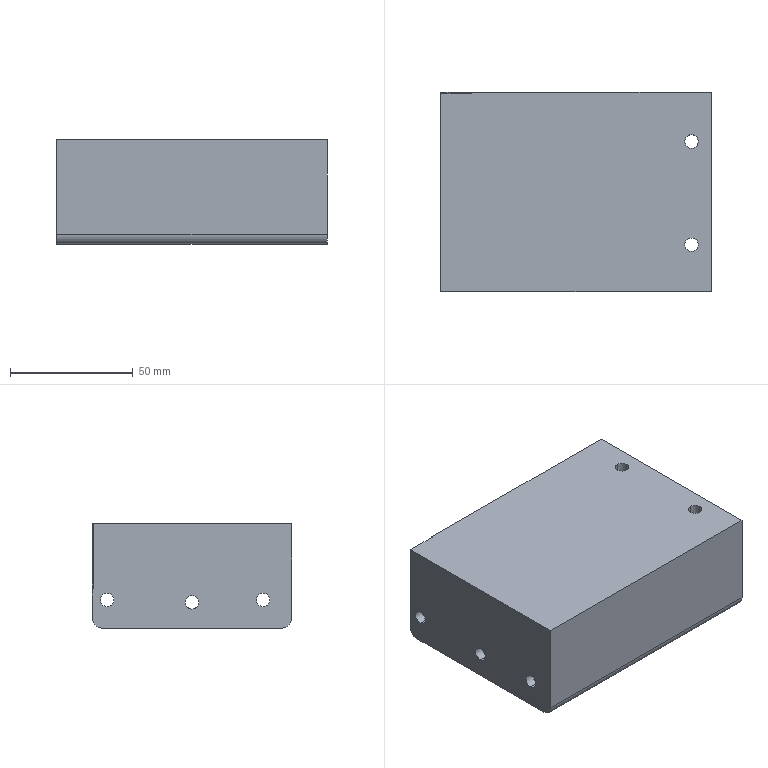Part | STEP file | FFH80-GY-002B^FFH85-PL-M75-B3-01_three-axis module | 1 solid | 46 faces | box 110 x 81 x 42.5 mm | volume 366642 mm3 | cylinder 29 | plane 15 | cone 2 | commonest cylinder face diameters 5.5 x10 9 x10 2.5 x2 3 x2 3.3 x2 8 x2
STEP:
#1=CARTESIAN_POINT('',(102.,23.25,21.25));
#2=VERTEX_POINT('',#1);
#3=CARTESIAN_POINT('',(102.,17.75,21.25));
#4=VERTEX_POINT('',#3);
#5=CARTESIAN_POINT('',(102.,20.5,21.25));
#6=DIRECTION('',(0.,0.,1.));
#7=DIRECTION('',(0.,1.,0.));
#8=AXIS2_PLACEMENT_3D('',#5,#6,#7);
#9=CIRCLE('',#8,2.75);
#10=EDGE_CURVE('',#2,#4,#9,.T.);
#11=ORIENTED_EDGE('',*,*,#10,.T.);
#12=CARTESIAN_POINT('',(102.,17.75,-15.25));
#13=VERTEX_POINT('',#12);
#14=CARTESIAN_POINT('',(102.,17.75,-21.25));
#15=DIRECTION('',(0.,0.,-1.));
#16=VECTOR('',#15,1000.);
#17=LINE('',#14,#16);
#18=EDGE_CURVE('',#4,#13,#17,.T.);
#19=ORIENTED_EDGE('',*,*,#18,.T.);
#20=CARTESIAN_POINT('',(102.,23.25,-15.25));
#21=VERTEX_POINT('',#20);
#22=CARTESIAN_POINT('',(102.,20.5,-15.25));
#23=DIRECTION('',(0.,0.,1.));
#24=DIRECTION('',(0.,1.,0.));
#25=AXIS2_PLACEMENT_3D('',#22,#23,#24);
#26=CIRCLE('',#25,2.75);
#27=EDGE_CURVE('',#21,#13,#26,.T.);
#28=ORIENTED_EDGE('',*,*,#27,.F.);
#29=CARTESIAN_POINT('',(102.,23.25,-21.25));
#30=DIRECTION('',(0.,0.,-1.));
#31=VECTOR('',#30,1000.);
#32=LINE('',#29,#31);
#33=EDGE_CURVE('',#2,#21,#32,.T.);
#34=ORIENTED_EDGE('',*,*,#33,.F.);
#35=EDGE_LOOP('',(#11,#19,#28,#34));
#36=FACE_OUTER_BOUND('',#35,.T.);
#37=CARTESIAN_POINT('',(102.,20.5,-21.25));
#38=DIRECTION('',(0.,0.,-1.));
#39=DIRECTION('',(0.,1.,0.));
#40=AXIS2_PLACEMENT_3D('',#37,#38,#39);
#41=CYLINDRICAL_SURFACE('',#40,2.75);
#42=ADVANCED_FACE('',(#36),#41,.F.);
#43=CARTESIAN_POINT('',(102.,-18.75,21.25));
#44=VERTEX_POINT('',#43);
#45=CARTESIAN_POINT('',(102.,-24.25,21.25));
#46=VERTEX_POINT('',#45);
#47=CARTESIAN_POINT('',(102.,-21.5,21.25));
#48=DIRECTION('',(0.,0.,1.));
#49=DIRECTION('',(0.,1.,0.));
#50=AXIS2_PLACEMENT_3D('',#47,#48,#49);
#51=CIRCLE('',#50,2.75);
#52=EDGE_CURVE('',#44,#46,#51,.T.);
#53=ORIENTED_EDGE('',*,*,#52,.T.);
#54=CARTESIAN_POINT('',(102.,-24.25,-15.25));
#55=VERTEX_POINT('',#54);
#56=CARTESIAN_POINT('',(102.,-24.25,-21.25));
#57=DIRECTION('',(0.,0.,-1.));
#58=VECTOR('',#57,1000.);
#59=LINE('',#56,#58);
#60=EDGE_CURVE('',#46,#55,#59,.T.);
#61=ORIENTED_EDGE('',*,*,#60,.T.);
#62=CARTESIAN_POINT('',(102.,-18.75,-15.25));
#63=VERTEX_POINT('',#62);
#64=CARTESIAN_POINT('',(102.,-21.5,-15.25));
#65=DIRECTION('',(0.,0.,1.));
#66=DIRECTION('',(0.,1.,0.));
#67=AXIS2_PLACEMENT_3D('',#64,#65,#66);
#68=CIRCLE('',#67,2.75);
#69=EDGE_CURVE('',#63,#55,#68,.T.);
#70=ORIENTED_EDGE('',*,*,#69,.F.);
#71=CARTESIAN_POINT('',(102.,-18.75,-21.25));
#72=DIRECTION('',(0.,0.,-1.));
#73=VECTOR('',#72,1000.);
#74=LINE('',#71,#73);
#75=EDGE_CURVE('',#44,#63,#74,.T.);
#76=ORIENTED_EDGE('',*,*,#75,.F.);
#77=EDGE_LOOP('',(#53,#61,#70,#76));
#78=FACE_OUTER_BOUND('',#77,.T.);
#79=CARTESIAN_POINT('',(102.,-21.5,-21.25));
#80=DIRECTION('',(0.,0.,-1.));
#81=DIRECTION('',(0.,1.,0.));
#82=AXIS2_PLACEMENT_3D('',#79,#80,#81);
#83=CYLINDRICAL_SURFACE('',#82,2.75);
#84=ADVANCED_FACE('',(#78),#83,.F.);
#85=CARTESIAN_POINT('',(6.,34.2,3.75));
#86=VERTEX_POINT('',#85);
#87=CARTESIAN_POINT('',(6.,34.2,6.75));
#88=VERTEX_POINT('',#87);
#89=CARTESIAN_POINT('',(6.,34.2,5.25));
#90=DIRECTION('',(0.,1.,0.));
#91=DIRECTION('',(0.,0.,1.));
#92=AXIS2_PLACEMENT_3D('',#89,#90,#91);
#93=CIRCLE('',#92,1.5);
#94=EDGE_CURVE('',#86,#88,#93,.T.);
#95=ORIENTED_EDGE('',*,*,#94,.F.);
#96=CARTESIAN_POINT('',(6.,40.2,3.75));
#97=VERTEX_POINT('',#96);
#98=CARTESIAN_POINT('',(6.,40.2,3.75));
#99=DIRECTION('',(0.,1.,0.));
#100=VECTOR('',#99,1000.);
#101=LINE('',#98,#100);
#102=EDGE_CURVE('',#86,#97,#101,.T.);
#103=ORIENTED_EDGE('',*,*,#102,.T.);
#104=CARTESIAN_POINT('',(6.,40.2,6.75));
#105=VERTEX_POINT('',#104);
#106=CARTESIAN_POINT('',(6.,40.2,5.25));
#107=DIRECTION('',(0.,1.,0.));
#108=DIRECTION('',(0.,0.,1.));
#109=AXIS2_PLACEMENT_3D('',#106,#107,#108);
#110=CIRCLE('',#109,1.5);
#111=EDGE_CURVE('',#97,#105,#110,.T.);
#112=ORIENTED_EDGE('',*,*,#111,.T.);
#113=CARTESIAN_POINT('',(6.,40.2,6.75));
#114=DIRECTION('',(0.,1.,0.));
#115=VECTOR('',#114,1000.);
#116=LINE('',#113,#115);
#117=EDGE_CURVE('',#88,#105,#116,.T.);
#118=ORIENTED_EDGE('',*,*,#117,.F.);
#119=EDGE_LOOP('',(#95,#103,#112,#118));
#120=FACE_OUTER_BOUND('',#119,.T.);
#121=CARTESIAN_POINT('',(6.,40.2,5.25));
#122=DIRECTION('',(0.,1.,0.));
#123=DIRECTION('',(0.,0.,1.));
#124=AXIS2_PLACEMENT_3D('',#121,#122,#123);
#125=CYLINDRICAL_SURFACE('',#124,1.5);
#126=ADVANCED_FACE('',(#120),#125,.F.);
#127=CARTESIAN_POINT('',(0.,0.,-8.));
#128=VERTEX_POINT('',#127);
#129=CARTESIAN_POINT('',(0.,0.,-13.5));
#130=VERTEX_POINT('',#129);
#131=CARTESIAN_POINT('',(0.,0.,-10.75));
#132=DIRECTION('',(1.,0.,0.));
#133=DIRECTION('',(0.,0.,-1.));
#134=AXIS2_PLACEMENT_3D('',#131,#132,#133);
#135=CIRCLE('',#134,2.75);
#136=EDGE_CURVE('',#128,#130,#135,.T.);
#137=ORIENTED_EDGE('',*,*,#136,.F.);
#138=CARTESIAN_POINT('',(104.,0.,-8.));
#139=VERTEX_POINT('',#138);
#140=CARTESIAN_POINT('',(110.,0.,-8.));
#141=DIRECTION('',(1.,0.,0.));
#142=VECTOR('',#141,1000.);
#143=LINE('',#140,#142);
#144=EDGE_CURVE('',#128,#139,#143,.T.);
#145=ORIENTED_EDGE('',*,*,#144,.T.);
#146=CARTESIAN_POINT('',(104.,0.,-13.5));
#147=VERTEX_POINT('',#146);
#148=CARTESIAN_POINT('',(104.,0.,-10.75));
#149=DIRECTION('',(-1.,0.,0.));
#150=DIRECTION('',(0.,0.,-1.));
#151=AXIS2_PLACEMENT_3D('',#148,#149,#150);
#152=CIRCLE('',#151,2.75);
#153=EDGE_CURVE('',#147,#139,#152,.T.);
#154=ORIENTED_EDGE('',*,*,#153,.F.);
#155=CARTESIAN_POINT('',(100.65,0.,-13.5));
#156=VERTEX_POINT('',#155);
#157=CARTESIAN_POINT('',(110.,0.,-13.5));
#158=DIRECTION('',(1.,0.,0.));
#159=VECTOR('',#158,1000.);
#160=LINE('',#157,#159);
#161=EDGE_CURVE('',#156,#147,#160,.T.);
#162=ORIENTED_EDGE('',*,*,#161,.F.);
#163=CARTESIAN_POINT('',(99.,-1.65,-12.95));
#164=VERTEX_POINT('',#163);
#165=CARTESIAN_POINT('',(99.,-1.65,-12.95));
#166=CARTESIAN_POINT('',(99.112,-1.65,-12.95));
#167=CARTESIAN_POINT('',(99.222,-1.639,-12.959));
#168=CARTESIAN_POINT('',(99.436,-1.595,-12.99));
#169=CARTESIAN_POINT('',(99.542,-1.562,-13.014));
#170=CARTESIAN_POINT('',(99.838,-1.437,-13.097));
#171=CARTESIAN_POINT('',(100.016,-1.317,-13.17));
#172=CARTESIAN_POINT('',(100.239,-1.094,-13.274));
#173=CARTESIAN_POINT('',(100.308,-1.012,-13.309));
#174=CARTESIAN_POINT('',(100.427,-0.8358,-13.372));
#175=CARTESIAN_POINT('',(100.477,-0.7424,-13.4));
#176=CARTESIAN_POINT('',(100.562,-0.5439,-13.448));
#177=CARTESIAN_POINT('',(100.595,-0.4374,-13.467));
#178=CARTESIAN_POINT('',(100.639,-0.222,-13.493));
#179=CARTESIAN_POINT('',(100.65,-0.1122,-13.5));
#180=CARTESIAN_POINT('',(100.65,0.,-13.5));
#181=B_SPLINE_CURVE_WITH_KNOTS('',3,(#165,#166,#167,#168,#169,#170,#171,#172,#173,#174,#175,#176,#177,#178,#179,#180),.UNSPECIFIED.,.F.,.F.,(4,2,2,2,2,2,2,4),(0.,0.0003309,0.0006617,0.001323,0.001654,0.001985,0.002316,0.002647),.UNSPECIFIED.);
#182=EDGE_CURVE('',#164,#156,#181,.T.);
#183=ORIENTED_EDGE('',*,*,#182,.F.);
#184=CARTESIAN_POINT('',(97.35,0.,-13.5));
#185=VERTEX_POINT('',#184);
#186=CARTESIAN_POINT('',(97.35,0.,-13.5));
#187=CARTESIAN_POINT('',(97.35,-0.1121,-13.5));
#188=CARTESIAN_POINT('',(97.361,-0.2218,-13.493));
#189=CARTESIAN_POINT('',(97.405,-0.4369,-13.467));
#190=CARTESIAN_POINT('',(97.438,-0.5432,-13.448));
#191=CARTESIAN_POINT('',(97.565,-0.842,-13.376));
#192=CARTESIAN_POINT('',(97.687,-1.021,-13.309));
#193=CARTESIAN_POINT('',(97.91,-1.243,-13.204));
#194=CARTESIAN_POINT('',(97.993,-1.311,-13.168));
#195=CARTESIAN_POINT('',(98.168,-1.429,-13.101));
#196=CARTESIAN_POINT('',(98.261,-1.479,-13.069));
#197=CARTESIAN_POINT('',(98.458,-1.562,-13.014));
#198=CARTESIAN_POINT('',(98.564,-1.595,-12.99));
#199=CARTESIAN_POINT('',(98.778,-1.639,-12.959));
#200=CARTESIAN_POINT('',(98.888,-1.65,-12.95));
#201=CARTESIAN_POINT('',(99.,-1.65,-12.95));
#202=B_SPLINE_CURVE_WITH_KNOTS('',3,(#186,#187,#188,#189,#190,#191,#192,#193,#194,#195,#196,#197,#198,#199,#200,#201),.UNSPECIFIED.,.F.,.F.,(4,2,2,2,2,2,2,4),(-0.002649,-0.002318,-0.001986,-0.001324,-0.0009932,-0.0006622,-0.0003311,0.),.UNSPECIFIED.);
#203=EDGE_CURVE('',#185,#164,#202,.T.);
#204=ORIENTED_EDGE('',*,*,#203,.F.);
#205=CARTESIAN_POINT('',(110.,0.,-13.5));
#206=DIRECTION('',(1.,0.,0.));
#207=VECTOR('',#206,1000.);
#208=LINE('',#205,#207);
#209=EDGE_CURVE('',#130,#185,#208,.T.);
#210=ORIENTED_EDGE('',*,*,#209,.F.);
#211=EDGE_LOOP('',(#137,#145,#154,#162,#183,#204,#210));
#212=FACE_OUTER_BOUND('',#211,.T.);
#213=CARTESIAN_POINT('',(110.,0.,-10.75));
#214=DIRECTION('',(1.,0.,0.));
#215=DIRECTION('',(0.,0.,-1.));
#216=AXIS2_PLACEMENT_3D('',#213,#214,#215);
#217=CYLINDRICAL_SURFACE('',#216,2.75);
#218=ADVANCED_FACE('',(#212),#217,.F.);
#219=CARTESIAN_POINT('',(0.,34.5,-7.));
#220=VERTEX_POINT('',#219);
#221=CARTESIAN_POINT('',(0.,34.5,-12.5));
#222=VERTEX_POINT('',#221);
#223=CARTESIAN_POINT('',(0.,34.5,-9.75));
#224=DIRECTION('',(1.,0.,0.));
#225=DIRECTION('',(0.,0.,-1.));
#226=AXIS2_PLACEMENT_3D('',#223,#224,#225);
#227=CIRCLE('',#226,2.75);
#228=EDGE_CURVE('',#220,#222,#227,.T.);
#229=ORIENTED_EDGE('',*,*,#228,.F.);
#230=CARTESIAN_POINT('',(104.,34.5,-7.));
#231=VERTEX_POINT('',#230);
#232=CARTESIAN_POINT('',(110.,34.5,-7.));
#233=DIRECTION('',(1.,0.,0.));
#234=VECTOR('',#233,1000.);
#235=LINE('',#232,#234);
#236=EDGE_CURVE('',#220,#231,#235,.T.);
#237=ORIENTED_EDGE('',*,*,#236,.T.);
#238=CARTESIAN_POINT('',(104.,34.5,-12.5));
#239=VERTEX_POINT('',#238);
#240=CARTESIAN_POINT('',(104.,34.5,-9.75));
#241=DIRECTION('',(-1.,0.,0.));
#242=DIRECTION('',(0.,0.,-1.));
#243=AXIS2_PLACEMENT_3D('',#240,#241,#242);
#244=CIRCLE('',#243,2.75);
#245=EDGE_CURVE('',#239,#231,#244,.T.);
#246=ORIENTED_EDGE('',*,*,#245,.F.);
#247=CARTESIAN_POINT('',(110.,34.5,-12.5));
#248=DIRECTION('',(1.,0.,0.));
#249=VECTOR('',#248,1000.);
#250=LINE('',#247,#249);
#251=EDGE_CURVE('',#222,#239,#250,.T.);
#252=ORIENTED_EDGE('',*,*,#251,.F.);
#253=EDGE_LOOP('',(#229,#237,#246,#252));
#254=FACE_OUTER_BOUND('',#253,.T.);
#255=CARTESIAN_POINT('',(110.,34.5,-9.75));
#256=DIRECTION('',(1.,0.,0.));
#257=DIRECTION('',(0.,0.,-1.));
#258=AXIS2_PLACEMENT_3D('',#255,#256,#257);
#259=CYLINDRICAL_SURFACE('',#258,2.75);
#260=ADVANCED_FACE('',(#254),#259,.F.);
#261=CARTESIAN_POINT('',(0.,-29.,-7.));
#262=VERTEX_POINT('',#261);
#263=CARTESIAN_POINT('',(0.,-29.,-12.5));
#264=VERTEX_POINT('',#263);
#265=CARTESIAN_POINT('',(0.,-29.,-9.75));
#266=DIRECTION('',(1.,0.,0.));
#267=DIRECTION('',(0.,0.,-1.));
#268=AXIS2_PLACEMENT_3D('',#265,#266,#267);
#269=CIRCLE('',#268,2.75);
#270=EDGE_CURVE('',#262,#264,#269,.T.);
#271=ORIENTED_EDGE('',*,*,#270,.F.);
#272=CARTESIAN_POINT('',(104.,-29.,-7.));
#273=VERTEX_POINT('',#272);
#274=CARTESIAN_POINT('',(110.,-29.,-7.));
#275=DIRECTION('',(1.,0.,0.));
#276=VECTOR('',#275,1000.);
#277=LINE('',#274,#276);
#278=EDGE_CURVE('',#262,#273,#277,.T.);
#279=ORIENTED_EDGE('',*,*,#278,.T.);
#280=CARTESIAN_POINT('',(104.,-29.,-12.5));
#281=VERTEX_POINT('',#280);
#282=CARTESIAN_POINT('',(104.,-29.,-9.75));
#283=DIRECTION('',(-1.,0.,0.));
#284=DIRECTION('',(0.,0.,-1.));
#285=AXIS2_PLACEMENT_3D('',#282,#283,#284);
#286=CIRCLE('',#285,2.75);
#287=EDGE_CURVE('',#281,#273,#286,.T.);
#288=ORIENTED_EDGE('',*,*,#287,.F.);
#289=CARTESIAN_POINT('',(110.,-29.,-12.5));
#290=DIRECTION('',(1.,0.,0.));
#291=VECTOR('',#290,1000.);
#292=LINE('',#289,#291);
#293=EDGE_CURVE('',#264,#281,#292,.T.);
#294=ORIENTED_EDGE('',*,*,#293,.F.);
#295=EDGE_LOOP('',(#271,#279,#288,#294));
#296=FACE_OUTER_BOUND('',#295,.T.);
#297=CARTESIAN_POINT('',(110.,-29.,-9.75));
#298=DIRECTION('',(1.,0.,0.));
#299=DIRECTION('',(0.,0.,-1.));
#300=AXIS2_PLACEMENT_3D('',#297,#298,#299);
#301=CYLINDRICAL_SURFACE('',#300,2.75);
#302=ADVANCED_FACE('',(#296),#301,.F.);
#303=CARTESIAN_POINT('',(104.,0.,-6.25));
#304=VERTEX_POINT('',#303);
#305=CARTESIAN_POINT('',(104.,0.,-15.25));
#306=VERTEX_POINT('',#305);
#307=CARTESIAN_POINT('',(104.,0.,-10.75));
#308=DIRECTION('',(1.,0.,0.));
#309=DIRECTION('',(0.,0.,-1.));
#310=AXIS2_PLACEMENT_3D('',#307,#308,#309);
#311=CIRCLE('',#310,4.5);
#312=EDGE_CURVE('',#304,#306,#311,.T.);
#313=ORIENTED_EDGE('',*,*,#312,.F.);
#314=CARTESIAN_POINT('',(110.,0.,-6.25));
#315=VERTEX_POINT('',#314);
#316=CARTESIAN_POINT('',(110.,0.,-6.25));
#317=DIRECTION('',(1.,0.,0.));
#318=VECTOR('',#317,1000.);
#319=LINE('',#316,#318);
#320=EDGE_CURVE('',#304,#315,#319,.T.);
#321=ORIENTED_EDGE('',*,*,#320,.T.);
#322=CARTESIAN_POINT('',(110.,0.,-15.25));
#323=VERTEX_POINT('',#322);
#324=CARTESIAN_POINT('',(110.,0.,-10.75));
#325=DIRECTION('',(1.,0.,0.));
#326=DIRECTION('',(0.,0.,-1.));
#327=AXIS2_PLACEMENT_3D('',#324,#325,#326);
#328=CIRCLE('',#327,4.5);
#329=EDGE_CURVE('',#315,#323,#328,.T.);
#330=ORIENTED_EDGE('',*,*,#329,.T.);
#331=CARTESIAN_POINT('',(110.,0.,-15.25));
#332=DIRECTION('',(1.,0.,0.));
#333=VECTOR('',#332,1000.);
#334=LINE('',#331,#333);
#335=EDGE_CURVE('',#306,#323,#334,.T.);
#336=ORIENTED_EDGE('',*,*,#335,.F.);
#337=EDGE_LOOP('',(#313,#321,#330,#336));
#338=FACE_OUTER_BOUND('',#337,.T.);
#339=CARTESIAN_POINT('',(110.,0.,-10.75));
#340=DIRECTION('',(1.,0.,0.));
#341=DIRECTION('',(0.,0.,-1.));
#342=AXIS2_PLACEMENT_3D('',#339,#340,#341);
#343=CYLINDRICAL_SURFACE('',#342,4.5);
#344=ADVANCED_FACE('',(#338),#343,.F.);
#345=CARTESIAN_POINT('',(104.,34.5,-5.25));
#346=VERTEX_POINT('',#345);
#347=CARTESIAN_POINT('',(104.,34.5,-14.25));
#348=VERTEX_POINT('',#347);
#349=CARTESIAN_POINT('',(104.,34.5,-9.75));
#350=DIRECTION('',(1.,0.,0.));
#351=DIRECTION('',(0.,0.,-1.));
#352=AXIS2_PLACEMENT_3D('',#349,#350,#351);
#353=CIRCLE('',#352,4.5);
#354=EDGE_CURVE('',#346,#348,#353,.T.);
#355=ORIENTED_EDGE('',*,*,#354,.F.);
#356=CARTESIAN_POINT('',(110.,34.5,-5.25));
#357=VERTEX_POINT('',#356);
#358=CARTESIAN_POINT('',(110.,34.5,-5.25));
#359=DIRECTION('',(1.,0.,0.));
#360=VECTOR('',#359,1000.);
#361=LINE('',#358,#360);
#362=EDGE_CURVE('',#346,#357,#361,.T.);
#363=ORIENTED_EDGE('',*,*,#362,.T.);
#364=CARTESIAN_POINT('',(110.,34.5,-14.25));
#365=VERTEX_POINT('',#364);
#366=CARTESIAN_POINT('',(110.,34.5,-9.75));
#367=DIRECTION('',(1.,0.,0.));
#368=DIRECTION('',(0.,0.,-1.));
#369=AXIS2_PLACEMENT_3D('',#366,#367,#368);
#370=CIRCLE('',#369,4.5);
#371=EDGE_CURVE('',#357,#365,#370,.T.);
#372=ORIENTED_EDGE('',*,*,#371,.T.);
#373=CARTESIAN_POINT('',(110.,34.5,-14.25));
#374=DIRECTION('',(1.,0.,0.));
#375=VECTOR('',#374,1000.);
#376=LINE('',#373,#375);
#377=EDGE_CURVE('',#348,#365,#376,.T.);
#378=ORIENTED_EDGE('',*,*,#377,.F.);
#379=EDGE_LOOP('',(#355,#363,#372,#378));
#380=FACE_OUTER_BOUND('',#379,.T.);
#381=CARTESIAN_POINT('',(110.,34.5,-9.75));
#382=DIRECTION('',(1.,0.,0.));
#383=DIRECTION('',(0.,0.,-1.));
#384=AXIS2_PLACEMENT_3D('',#381,#382,#383);
#385=CYLINDRICAL_SURFACE('',#384,4.5);
#386=ADVANCED_FACE('',(#380),#385,.F.);
#387=CARTESIAN_POINT('',(104.,-29.,-5.25));
#388=VERTEX_POINT('',#387);
#389=CARTESIAN_POINT('',(104.,-29.,-14.25));
#390=VERTEX_POINT('',#389);
#391=CARTESIAN_POINT('',(104.,-29.,-9.75));
#392=DIRECTION('',(1.,0.,0.));
#393=DIRECTION('',(0.,0.,-1.));
#394=AXIS2_PLACEMENT_3D('',#391,#392,#393);
#395=CIRCLE('',#394,4.5);
#396=EDGE_CURVE('',#388,#390,#395,.T.);
#397=ORIENTED_EDGE('',*,*,#396,.F.);
#398=CARTESIAN_POINT('',(110.,-29.,-5.25));
#399=VERTEX_POINT('',#398);
#400=CARTESIAN_POINT('',(110.,-29.,-5.25));
#401=DIRECTION('',(1.,0.,0.));
#402=VECTOR('',#401,1000.);
#403=LINE('',#400,#402);
#404=EDGE_CURVE('',#388,#399,#403,.T.);
#405=ORIENTED_EDGE('',*,*,#404,.T.);
#406=CARTESIAN_POINT('',(110.,-29.,-14.25));
#407=VERTEX_POINT('',#406);
#408=CARTESIAN_POINT('',(110.,-29.,-9.75));
#409=DIRECTION('',(1.,0.,0.));
#410=DIRECTION('',(0.,0.,-1.));
#411=AXIS2_PLACEMENT_3D('',#408,#409,#410);
#412=CIRCLE('',#411,4.5);
#413=EDGE_CURVE('',#399,#407,#412,.T.);
#414=ORIENTED_EDGE('',*,*,#413,.T.);
#415=CARTESIAN_POINT('',(110.,-29.,-14.25));
#416=DIRECTION('',(1.,0.,0.));
#417=VECTOR('',#416,1000.);
#418=LINE('',#415,#417);
#419=EDGE_CURVE('',#390,#407,#418,.T.);
#420=ORIENTED_EDGE('',*,*,#419,.F.);
#421=EDGE_LOOP('',(#397,#405,#414,#420));
#422=FACE_OUTER_BOUND('',#421,.T.);
#423=CARTESIAN_POINT('',(110.,-29.,-9.75));
#424=DIRECTION('',(1.,0.,0.));
#425=DIRECTION('',(0.,0.,-1.));
#426=AXIS2_PLACEMENT_3D('',#423,#424,#425);
#427=CYLINDRICAL_SURFACE('',#426,4.5);
#428=ADVANCED_FACE('',(#422),#427,.F.);
#429=CARTESIAN_POINT('',(102.,25.,-15.25));
#430=VERTEX_POINT('',#429);
#431=CARTESIAN_POINT('',(102.,16.,-15.25));
#432=VERTEX_POINT('',#431);
#433=CARTESIAN_POINT('',(102.,20.5,-15.25));
#434=DIRECTION('',(0.,0.,1.));
#435=DIRECTION('',(0.,1.,0.));
#436=AXIS2_PLACEMENT_3D('',#433,#434,#435);
#437=CIRCLE('',#436,4.5);
#438=EDGE_CURVE('',#430,#432,#437,.T.);
#439=ORIENTED_EDGE('',*,*,#438,.T.);
#440=CARTESIAN_POINT('',(102.,16.,-21.25));
#441=VERTEX_POINT('',#440);
#442=CARTESIAN_POINT('',(102.,16.,-21.25));
#443=DIRECTION('',(0.,0.,-1.));
#444=VECTOR('',#443,1000.);
#445=LINE('',#442,#444);
#446=EDGE_CURVE('',#432,#441,#445,.T.);
#447=ORIENTED_EDGE('',*,*,#446,.T.);
#448=CARTESIAN_POINT('',(102.,25.,-21.25));
#449=VERTEX_POINT('',#448);
#450=CARTESIAN_POINT('',(102.,20.5,-21.25));
#451=DIRECTION('',(0.,0.,-1.));
#452=DIRECTION('',(0.,1.,0.));
#453=AXIS2_PLACEMENT_3D('',#450,#451,#452);
#454=CIRCLE('',#453,4.5);
#455=EDGE_CURVE('',#441,#449,#454,.T.);
#456=ORIENTED_EDGE('',*,*,#455,.T.);
#457=CARTESIAN_POINT('',(102.,25.,-21.25));
#458=DIRECTION('',(0.,0.,-1.));
#459=VECTOR('',#458,1000.);
#460=LINE('',#457,#459);
#461=EDGE_CURVE('',#430,#449,#460,.T.);
#462=ORIENTED_EDGE('',*,*,#461,.F.);
#463=EDGE_LOOP('',(#439,#447,#456,#462));
#464=FACE_OUTER_BOUND('',#463,.T.);
#465=CARTESIAN_POINT('',(102.,20.5,-21.25));
#466=DIRECTION('',(0.,0.,-1.));
#467=DIRECTION('',(0.,1.,0.));
#468=AXIS2_PLACEMENT_3D('',#465,#466,#467);
#469=CYLINDRICAL_SURFACE('',#468,4.5);
#470=ADVANCED_FACE('',(#464),#469,.F.);
#471=CARTESIAN_POINT('',(102.,-17.,-15.25));
#472=VERTEX_POINT('',#471);
#473=CARTESIAN_POINT('',(102.,-26.,-15.25));
#474=VERTEX_POINT('',#473);
#475=CARTESIAN_POINT('',(102.,-21.5,-15.25));
#476=DIRECTION('',(0.,0.,1.));
#477=DIRECTION('',(0.,1.,0.));
#478=AXIS2_PLACEMENT_3D('',#475,#476,#477);
#479=CIRCLE('',#478,4.5);
#480=EDGE_CURVE('',#472,#474,#479,.T.);
#481=ORIENTED_EDGE('',*,*,#480,.T.);
#482=CARTESIAN_POINT('',(102.,-26.,-21.25));
#483=VERTEX_POINT('',#482);
#484=CARTESIAN_POINT('',(102.,-26.,-21.25));
#485=DIRECTION('',(0.,0.,-1.));
#486=VECTOR('',#485,1000.);
#487=LINE('',#484,#486);
#488=EDGE_CURVE('',#474,#483,#487,.T.);
#489=ORIENTED_EDGE('',*,*,#488,.T.);
#490=CARTESIAN_POINT('',(102.,-17.,-21.25));
#491=VERTEX_POINT('',#490);
#492=CARTESIAN_POINT('',(102.,-21.5,-21.25));
#493=DIRECTION('',(0.,0.,-1.));
#494=DIRECTION('',(0.,1.,0.));
#495=AXIS2_PLACEMENT_3D('',#492,#493,#494);
#496=CIRCLE('',#495,4.5);
#497=EDGE_CURVE('',#483,#491,#496,.T.);
#498=ORIENTED_EDGE('',*,*,#497,.T.);
#499=CARTESIAN_POINT('',(102.,-17.,-21.25));
#500=DIRECTION('',(0.,0.,-1.));
#501=VECTOR('',#500,1000.);
#502=LINE('',#499,#501);
#503=EDGE_CURVE('',#472,#491,#502,.T.);
#504=ORIENTED_EDGE('',*,*,#503,.F.);
#505=EDGE_LOOP('',(#481,#489,#498,#504));
#506=FACE_OUTER_BOUND('',#505,.T.);
#507=CARTESIAN_POINT('',(102.,-21.5,-21.25));
#508=DIRECTION('',(0.,0.,-1.));
#509=DIRECTION('',(0.,1.,0.));
#510=AXIS2_PLACEMENT_3D('',#507,#508,#509);
#511=CYLINDRICAL_SURFACE('',#510,4.5);
#512=ADVANCED_FACE('',(#506),#511,.F.);
#513=CARTESIAN_POINT('',(99.,1.65,-12.95));
#514=VERTEX_POINT('',#513);
#515=CARTESIAN_POINT('',(99.,1.65,-12.95));
#516=CARTESIAN_POINT('',(98.888,1.65,-12.95));
#517=CARTESIAN_POINT('',(98.778,1.639,-12.959));
#518=CARTESIAN_POINT('',(98.564,1.595,-12.99));
#519=CARTESIAN_POINT('',(98.458,1.562,-13.014));
#520=CARTESIAN_POINT('',(98.162,1.437,-13.097));
#521=CARTESIAN_POINT('',(97.984,1.317,-13.17));
#522=CARTESIAN_POINT('',(97.761,1.094,-13.274));
#523=CARTESIAN_POINT('',(97.692,1.012,-13.309));
#524=CARTESIAN_POINT('',(97.573,0.8358,-13.372));
#525=CARTESIAN_POINT('',(97.523,0.7424,-13.4));
#526=CARTESIAN_POINT('',(97.438,0.5439,-13.448));
#527=CARTESIAN_POINT('',(97.405,0.4374,-13.467));
#528=CARTESIAN_POINT('',(97.361,0.222,-13.493));
#529=CARTESIAN_POINT('',(97.35,0.1119,-13.5));
#530=CARTESIAN_POINT('',(97.35,0.,-13.5));
#531=B_SPLINE_CURVE_WITH_KNOTS('',3,(#515,#516,#517,#518,#519,#520,#521,#522,#523,#524,#525,#526,#527,#528,#529,#530),.UNSPECIFIED.,.F.,.F.,(4,2,2,2,2,2,2,4),(0.005292,0.005622,0.005953,0.006614,0.006944,0.007274,0.007605,0.007935),.UNSPECIFIED.);
#532=EDGE_CURVE('',#514,#185,#531,.T.);
#533=ORIENTED_EDGE('',*,*,#532,.T.);
#534=ORIENTED_EDGE('',*,*,#203,.T.);
#535=CARTESIAN_POINT('',(99.,-1.65,-21.25));
#536=VERTEX_POINT('',#535);
#537=CARTESIAN_POINT('',(99.,-1.65,-21.25));
#538=DIRECTION('',(0.,0.,-1.));
#539=VECTOR('',#538,1000.);
#540=LINE('',#537,#539);
#541=EDGE_CURVE('',#164,#536,#540,.T.);
#542=ORIENTED_EDGE('',*,*,#541,.T.);
#543=CARTESIAN_POINT('',(99.,1.65,-21.25));
#544=VERTEX_POINT('',#543);
#545=CARTESIAN_POINT('',(99.,0.,-21.25));
#546=DIRECTION('',(0.,0.,-1.));
#547=DIRECTION('',(0.,1.,0.));
#548=AXIS2_PLACEMENT_3D('',#545,#546,#547);
#549=CIRCLE('',#548,1.65);
#550=EDGE_CURVE('',#536,#544,#549,.T.);
#551=ORIENTED_EDGE('',*,*,#550,.T.);
#552=CARTESIAN_POINT('',(99.,1.65,-21.25));
#553=DIRECTION('',(0.,0.,-1.));
#554=VECTOR('',#553,1000.);
#555=LINE('',#552,#554);
#556=EDGE_CURVE('',#514,#544,#555,.T.);
#557=ORIENTED_EDGE('',*,*,#556,.F.);
#558=EDGE_LOOP('',(#533,#534,#542,#551,#557));
#559=FACE_OUTER_BOUND('',#558,.T.);
#560=CARTESIAN_POINT('',(99.,0.,-21.25));
#561=DIRECTION('',(0.,0.,-1.));
#562=DIRECTION('',(0.,1.,0.));
#563=AXIS2_PLACEMENT_3D('',#560,#561,#562);
#564=CYLINDRICAL_SURFACE('',#563,1.65);
#565=ADVANCED_FACE('',(#559),#564,.F.);
#566=CARTESIAN_POINT('',(6.,31.7,4.));
#567=VERTEX_POINT('',#566);
#568=CARTESIAN_POINT('',(6.,31.7,6.5));
#569=VERTEX_POINT('',#568);
#570=CARTESIAN_POINT('',(6.,31.7,5.25));
#571=DIRECTION('',(0.,1.,0.));
#572=DIRECTION('',(0.,0.,1.));
#573=AXIS2_PLACEMENT_3D('',#570,#571,#572);
#574=CIRCLE('',#573,1.25);
#575=EDGE_CURVE('',#567,#569,#574,.T.);
#576=ORIENTED_EDGE('',*,*,#575,.F.);
#577=CARTESIAN_POINT('',(6.,34.2,4.));
#578=VERTEX_POINT('',#577);
#579=CARTESIAN_POINT('',(6.,40.2,4.));
#580=DIRECTION('',(0.,1.,0.));
#581=VECTOR('',#580,1000.);
#582=LINE('',#579,#581);
#583=EDGE_CURVE('',#567,#578,#582,.T.);
#584=ORIENTED_EDGE('',*,*,#583,.T.);
#585=CARTESIAN_POINT('',(6.,34.2,6.5));
#586=VERTEX_POINT('',#585);
#587=CARTESIAN_POINT('',(6.,34.2,5.25));
#588=DIRECTION('',(0.,1.,0.));
#589=DIRECTION('',(0.,0.,1.));
#590=AXIS2_PLACEMENT_3D('',#587,#588,#589);
#591=CIRCLE('',#590,1.25);
#592=EDGE_CURVE('',#578,#586,#591,.T.);
#593=ORIENTED_EDGE('',*,*,#592,.T.);
#594=CARTESIAN_POINT('',(6.,40.2,6.5));
#595=DIRECTION('',(0.,1.,0.));
#596=VECTOR('',#595,1000.);
#597=LINE('',#594,#596);
#598=EDGE_CURVE('',#569,#586,#597,.T.);
#599=ORIENTED_EDGE('',*,*,#598,.F.);
#600=EDGE_LOOP('',(#576,#584,#593,#599));
#601=FACE_OUTER_BOUND('',#600,.T.);
#602=CARTESIAN_POINT('',(6.,40.2,5.25));
#603=DIRECTION('',(0.,1.,0.));
#604=DIRECTION('',(0.,0.,1.));
#605=AXIS2_PLACEMENT_3D('',#602,#603,#604);
#606=CYLINDRICAL_SURFACE('',#605,1.25);
#607=ADVANCED_FACE('',(#601),#606,.F.);
#608=CARTESIAN_POINT('',(6.,30.949,5.25));
#609=VERTEX_POINT('',#608);
#610=CARTESIAN_POINT('',(6.,31.7,6.5));
#611=DIRECTION('',(0.,0.515,0.8572));
#612=VECTOR('',#611,1000.);
#613=LINE('',#610,#612);
#614=EDGE_CURVE('',#609,#569,#613,.T.);
#615=ORIENTED_EDGE('',*,*,#614,.F.);
#616=CARTESIAN_POINT('',(6.,31.7,4.));
#617=DIRECTION('',(0.,0.515,-0.8572));
#618=VECTOR('',#617,1000.);
#619=LINE('',#616,#618);
#620=EDGE_CURVE('',#609,#567,#619,.T.);
#621=ORIENTED_EDGE('',*,*,#620,.T.);
#622=ORIENTED_EDGE('',*,*,#575,.T.);
#623=EDGE_LOOP('',(#615,#621,#622));
#624=FACE_OUTER_BOUND('',#623,.T.);
#625=CARTESIAN_POINT('',(6.,31.7,5.25));
#626=DIRECTION('',(0.,1.,0.));
#627=DIRECTION('',(0.,0.,1.));
#628=AXIS2_PLACEMENT_3D('',#625,#626,#627);
#629=CONICAL_SURFACE('',#628,1.25,1.03);
#630=ADVANCED_FACE('',(#624),#629,.F.);
#631=ORIENTED_EDGE('',*,*,#10,.F.);
#632=CARTESIAN_POINT('',(102.,20.5,21.25));
#633=DIRECTION('',(0.,0.,1.));
#634=DIRECTION('',(0.,1.,0.));
#635=AXIS2_PLACEMENT_3D('',#632,#633,#634);
#636=CIRCLE('',#635,2.75);
#637=EDGE_CURVE('',#4,#2,#636,.T.);
#638=ORIENTED_EDGE('',*,*,#637,.F.);
#639=EDGE_LOOP('',(#631,#638));
#640=FACE_BOUND('',#639,.T.);
#641=ORIENTED_EDGE('',*,*,#52,.F.);
#642=CARTESIAN_POINT('',(102.,-21.5,21.25));
#643=DIRECTION('',(0.,0.,1.));
#644=DIRECTION('',(0.,1.,0.));
#645=AXIS2_PLACEMENT_3D('',#642,#643,#644);
#646=CIRCLE('',#645,2.75);
#647=EDGE_CURVE('',#46,#44,#646,.T.);
#648=ORIENTED_EDGE('',*,*,#647,.F.);
#649=EDGE_LOOP('',(#641,#648));
#650=FACE_BOUND('',#649,.T.);
#651=CARTESIAN_POINT('',(0.,40.2,21.25));
#652=VERTEX_POINT('',#651);
#653=CARTESIAN_POINT('',(12.5,40.2,21.25));
#654=VERTEX_POINT('',#653);
#655=CARTESIAN_POINT('',(110.,40.2,21.25));
#656=DIRECTION('',(1.,0.,0.));
#657=VECTOR('',#656,1000.);
#658=LINE('',#655,#657);
#659=EDGE_CURVE('',#652,#654,#658,.T.);
#660=ORIENTED_EDGE('',*,*,#659,.F.);
#661=CARTESIAN_POINT('',(0.,-40.5,21.25));
#662=VERTEX_POINT('',#661);
#663=CARTESIAN_POINT('',(0.,40.5,21.25));
#664=DIRECTION('',(0.,1.,0.));
#665=VECTOR('',#664,1000.);
#666=LINE('',#663,#665);
#667=EDGE_CURVE('',#662,#652,#666,.T.);
#668=ORIENTED_EDGE('',*,*,#667,.F.);
#669=CARTESIAN_POINT('',(110.,-40.5,21.25));
#670=VERTEX_POINT('',#669);
#671=CARTESIAN_POINT('',(110.,-40.5,21.25));
#672=DIRECTION('',(-1.,0.,0.));
#673=VECTOR('',#672,1000.);
#674=LINE('',#671,#673);
#675=EDGE_CURVE('',#670,#662,#674,.T.);
#676=ORIENTED_EDGE('',*,*,#675,.F.);
#677=CARTESIAN_POINT('',(110.,40.5,21.25));
#678=VERTEX_POINT('',#677);
#679=CARTESIAN_POINT('',(110.,40.5,21.25));
#680=DIRECTION('',(0.,-1.,0.));
#681=VECTOR('',#680,1000.);
#682=LINE('',#679,#681);
#683=EDGE_CURVE('',#678,#670,#682,.T.);
#684=ORIENTED_EDGE('',*,*,#683,.F.);
#685=CARTESIAN_POINT('',(12.5,40.5,21.25));
#686=VERTEX_POINT('',#685);
#687=CARTESIAN_POINT('',(110.,40.5,21.25));
#688=DIRECTION('',(1.,0.,0.));
#689=VECTOR('',#688,1000.);
#690=LINE('',#687,#689);
#691=EDGE_CURVE('',#686,#678,#690,.T.);
#692=ORIENTED_EDGE('',*,*,#691,.F.);
#693=CARTESIAN_POINT('',(12.5,40.2,21.25));
#694=DIRECTION('',(0.,-1.,0.));
#695=VECTOR('',#694,1000.);
#696=LINE('',#693,#695);
#697=EDGE_CURVE('',#686,#654,#696,.T.);
#698=ORIENTED_EDGE('',*,*,#697,.T.);
#699=EDGE_LOOP('',(#660,#668,#676,#684,#692,#698));
#700=FACE_OUTER_BOUND('',#699,.T.);
#701=CARTESIAN_POINT('',(110.,40.5,21.25));
#702=DIRECTION('',(0.,0.,-1.));
#703=DIRECTION('',(-1.,0.,0.));
#704=AXIS2_PLACEMENT_3D('',#701,#702,#703);
#705=PLANE('',#704);
#706=ADVANCED_FACE('',(#640,#650,#700),#705,.F.);
#707=ORIENTED_EDGE('',*,*,#18,.F.);
#708=ORIENTED_EDGE('',*,*,#637,.T.);
#709=ORIENTED_EDGE('',*,*,#33,.T.);
#710=CARTESIAN_POINT('',(102.,20.5,-15.25));
#711=DIRECTION('',(0.,0.,1.));
#712=DIRECTION('',(0.,1.,0.));
#713=AXIS2_PLACEMENT_3D('',#710,#711,#712);
#714=CIRCLE('',#713,2.75);
#715=EDGE_CURVE('',#13,#21,#714,.T.);
#716=ORIENTED_EDGE('',*,*,#715,.F.);
#717=EDGE_LOOP('',(#707,#708,#709,#716));
#718=FACE_OUTER_BOUND('',#717,.T.);
#719=CARTESIAN_POINT('',(102.,20.5,-21.25));
#720=DIRECTION('',(0.,0.,-1.));
#721=DIRECTION('',(0.,1.,0.));
#722=AXIS2_PLACEMENT_3D('',#719,#720,#721);
#723=CYLINDRICAL_SURFACE('',#722,2.75);
#724=ADVANCED_FACE('',(#718),#723,.F.);
#725=ORIENTED_EDGE('',*,*,#60,.F.);
#726=ORIENTED_EDGE('',*,*,#647,.T.);
#727=ORIENTED_EDGE('',*,*,#75,.T.);
#728=CARTESIAN_POINT('',(102.,-21.5,-15.25));
#729=DIRECTION('',(0.,0.,1.));
#730=DIRECTION('',(0.,1.,0.));
#731=AXIS2_PLACEMENT_3D('',#728,#729,#730);
#732=CIRCLE('',#731,2.75);
#733=EDGE_CURVE('',#55,#63,#732,.T.);
#734=ORIENTED_EDGE('',*,*,#733,.F.);
#735=EDGE_LOOP('',(#725,#726,#727,#734));
#736=FACE_OUTER_BOUND('',#735,.T.);
#737=CARTESIAN_POINT('',(102.,-21.5,-21.25));
#738=DIRECTION('',(0.,0.,-1.));
#739=DIRECTION('',(0.,1.,0.));
#740=AXIS2_PLACEMENT_3D('',#737,#738,#739);
#741=CYLINDRICAL_SURFACE('',#740,2.75);
#742=ADVANCED_FACE('',(#736),#741,.F.);
#743=CARTESIAN_POINT('',(6.,40.2,5.25));
#744=DIRECTION('',(0.,1.,0.));
#745=DIRECTION('',(0.,0.,1.));
#746=AXIS2_PLACEMENT_3D('',#743,#744,#745);
#747=CIRCLE('',#746,1.5);
#748=EDGE_CURVE('',#105,#97,#747,.T.);
#749=ORIENTED_EDGE('',*,*,#748,.F.);
#750=ORIENTED_EDGE('',*,*,#111,.F.);
#751=EDGE_LOOP('',(#749,#750));
#752=FACE_BOUND('',#751,.T.);
#753=CARTESIAN_POINT('',(0.,40.2,-5.25));
#754=VERTEX_POINT('',#753);
#755=CARTESIAN_POINT('',(10.5,40.2,-5.25));
#756=VERTEX_POINT('',#755);
#757=CARTESIAN_POINT('',(0.,40.2,-5.25));
#758=DIRECTION('',(1.,0.,0.));
#759=VECTOR('',#758,1000.);
#760=LINE('',#757,#759);
#761=EDGE_CURVE('',#754,#756,#760,.T.);
#762=ORIENTED_EDGE('',*,*,#761,.F.);
#763=CARTESIAN_POINT('',(0.,40.2,0.));
#764=DIRECTION('',(0.,0.,-1.));
#765=VECTOR('',#764,1000.);
#766=LINE('',#763,#765);
#767=EDGE_CURVE('',#652,#754,#766,.T.);
#768=ORIENTED_EDGE('',*,*,#767,.F.);
#769=ORIENTED_EDGE('',*,*,#659,.T.);
#770=CARTESIAN_POINT('',(12.5,40.2,-3.25));
#771=VERTEX_POINT('',#770);
#772=CARTESIAN_POINT('',(12.5,40.2,0.));
#773=DIRECTION('',(0.,0.,1.));
#774=VECTOR('',#773,1000.);
#775=LINE('',#772,#774);
#776=EDGE_CURVE('',#771,#654,#775,.T.);
#777=ORIENTED_EDGE('',*,*,#776,.F.);
#778=CARTESIAN_POINT('',(10.5,40.2,-3.25));
#779=DIRECTION('',(0.,-1.,0.));
#780=DIRECTION('',(0.,0.,-1.));
#781=AXIS2_PLACEMENT_3D('',#778,#779,#780);
#782=CIRCLE('',#781,2.);
#783=EDGE_CURVE('',#756,#771,#782,.T.);
#784=ORIENTED_EDGE('',*,*,#783,.F.);
#785=EDGE_LOOP('',(#762,#768,#769,#777,#784));
#786=FACE_OUTER_BOUND('',#785,.T.);
#787=CARTESIAN_POINT('',(0.,40.2,0.));
#788=DIRECTION('',(0.,-1.,0.));
#789=DIRECTION('',(0.,0.,-1.));
#790=AXIS2_PLACEMENT_3D('',#787,#788,#789);
#791=PLANE('',#790);
#792=ADVANCED_FACE('',(#752,#786),#791,.F.);
#793=CARTESIAN_POINT('',(0.,-36.5,-21.25));
#794=VERTEX_POINT('',#793);
#795=CARTESIAN_POINT('',(0.,-40.5,-17.25));
#796=VERTEX_POINT('',#795);
#797=CARTESIAN_POINT('',(0.,-36.5,-17.25));
#798=DIRECTION('',(-1.,0.,0.));
#799=DIRECTION('',(0.,0.,1.));
#800=AXIS2_PLACEMENT_3D('',#797,#798,#799);
#801=CIRCLE('',#800,4.);
#802=EDGE_CURVE('',#794,#796,#801,.T.);
#803=ORIENTED_EDGE('',*,*,#802,.T.);
#804=CARTESIAN_POINT('',(0.,-40.5,0.));
#805=DIRECTION('',(0.,0.,1.));
#806=VECTOR('',#805,1000.);
#807=LINE('',#804,#806);
#808=EDGE_CURVE('',#796,#662,#807,.T.);
#809=ORIENTED_EDGE('',*,*,#808,.T.);
#810=ORIENTED_EDGE('',*,*,#667,.T.);
#811=ORIENTED_EDGE('',*,*,#767,.T.);
#812=CARTESIAN_POINT('',(0.,40.5,-5.25));
#813=VERTEX_POINT('',#812);
#814=CARTESIAN_POINT('',(0.,0.,-5.25));
#815=DIRECTION('',(0.,1.,0.));
#816=VECTOR('',#815,1000.);
#817=LINE('',#814,#816);
#818=EDGE_CURVE('',#754,#813,#817,.T.);
#819=ORIENTED_EDGE('',*,*,#818,.T.);
#820=CARTESIAN_POINT('',(0.,40.5,-17.25));
#821=VERTEX_POINT('',#820);
#822=CARTESIAN_POINT('',(0.,40.5,0.));
#823=DIRECTION('',(0.,0.,-1.));
#824=VECTOR('',#823,1000.);
#825=LINE('',#822,#824);
#826=EDGE_CURVE('',#813,#821,#825,.T.);
#827=ORIENTED_EDGE('',*,*,#826,.T.);
#828=CARTESIAN_POINT('',(0.,36.5,-21.25));
#829=VERTEX_POINT('',#828);
#830=CARTESIAN_POINT('',(0.,36.5,-17.25));
#831=DIRECTION('',(-1.,0.,0.));
#832=DIRECTION('',(0.,0.,1.));
#833=AXIS2_PLACEMENT_3D('',#830,#831,#832);
#834=CIRCLE('',#833,4.);
#835=EDGE_CURVE('',#821,#829,#834,.T.);
#836=ORIENTED_EDGE('',*,*,#835,.T.);
#837=CARTESIAN_POINT('',(0.,0.,-21.25));
#838=DIRECTION('',(0.,-1.,0.));
#839=VECTOR('',#838,1000.);
#840=LINE('',#837,#839);
#841=EDGE_CURVE('',#829,#794,#840,.T.);
#842=ORIENTED_EDGE('',*,*,#841,.T.);
#843=EDGE_LOOP('',(#803,#809,#810,#811,#819,#827,#836,#842));
#844=FACE_OUTER_BOUND('',#843,.T.);
#845=CARTESIAN_POINT('',(0.,0.,-10.75));
#846=DIRECTION('',(1.,0.,0.));
#847=DIRECTION('',(0.,0.,-1.));
#848=AXIS2_PLACEMENT_3D('',#845,#846,#847);
#849=CIRCLE('',#848,2.75);
#850=EDGE_CURVE('',#130,#128,#849,.T.);
#851=ORIENTED_EDGE('',*,*,#850,.T.);
#852=ORIENTED_EDGE('',*,*,#136,.T.);
#853=EDGE_LOOP('',(#851,#852));
#854=FACE_BOUND('',#853,.T.);
#855=CARTESIAN_POINT('',(0.,34.5,-9.75));
#856=DIRECTION('',(1.,0.,0.));
#857=DIRECTION('',(0.,0.,-1.));
#858=AXIS2_PLACEMENT_3D('',#855,#856,#857);
#859=CIRCLE('',#858,2.75);
#860=EDGE_CURVE('',#222,#220,#859,.T.);
#861=ORIENTED_EDGE('',*,*,#860,.T.);
#862=ORIENTED_EDGE('',*,*,#228,.T.);
#863=EDGE_LOOP('',(#861,#862));
#864=FACE_BOUND('',#863,.T.);
#865=CARTESIAN_POINT('',(0.,-29.,-9.75));
#866=DIRECTION('',(1.,0.,0.));
#867=DIRECTION('',(0.,0.,-1.));
#868=AXIS2_PLACEMENT_3D('',#865,#866,#867);
#869=CIRCLE('',#868,2.75);
#870=EDGE_CURVE('',#264,#262,#869,.T.);
#871=ORIENTED_EDGE('',*,*,#870,.T.);
#872=ORIENTED_EDGE('',*,*,#270,.T.);
#873=EDGE_LOOP('',(#871,#872));
#874=FACE_BOUND('',#873,.T.);
#875=CARTESIAN_POINT('',(0.,0.,0.));
#876=DIRECTION('',(-1.,0.,0.));
#877=DIRECTION('',(0.,0.,1.));
#878=AXIS2_PLACEMENT_3D('',#875,#876,#877);
#879=PLANE('',#878);
#880=ADVANCED_FACE('',(#844,#854,#864,#874),#879,.T.);
#881=CARTESIAN_POINT('',(110.,-40.5,-17.25));
#882=VERTEX_POINT('',#881);
#883=CARTESIAN_POINT('',(110.,-40.5,-21.25));
#884=DIRECTION('',(0.,0.,-1.));
#885=VECTOR('',#884,1000.);
#886=LINE('',#883,#885);
#887=EDGE_CURVE('',#670,#882,#886,.T.);
#888=ORIENTED_EDGE('',*,*,#887,.F.);
#889=ORIENTED_EDGE('',*,*,#675,.T.);
#890=ORIENTED_EDGE('',*,*,#808,.F.);
#891=CARTESIAN_POINT('',(110.,-40.5,-17.25));
#892=DIRECTION('',(-1.,0.,0.));
#893=VECTOR('',#892,1000.);
#894=LINE('',#891,#893);
#895=EDGE_CURVE('',#882,#796,#894,.T.);
#896=ORIENTED_EDGE('',*,*,#895,.F.);
#897=EDGE_LOOP('',(#888,#889,#890,#896));
#898=FACE_OUTER_BOUND('',#897,.T.);
#899=CARTESIAN_POINT('',(110.,-40.5,-21.25));
#900=DIRECTION('',(0.,1.,0.));
#901=DIRECTION('',(0.,0.,1.));
#902=AXIS2_PLACEMENT_3D('',#899,#900,#901);
#903=PLANE('',#902);
#904=ADVANCED_FACE('',(#898),#903,.F.);
#905=CARTESIAN_POINT('',(110.,0.,-10.75));
#906=DIRECTION('',(1.,0.,0.));
#907=DIRECTION('',(0.,0.,-1.));
#908=AXIS2_PLACEMENT_3D('',#905,#906,#907);
#909=CIRCLE('',#908,4.5);
#910=EDGE_CURVE('',#323,#315,#909,.T.);
#911=ORIENTED_EDGE('',*,*,#910,.F.);
#912=ORIENTED_EDGE('',*,*,#329,.F.);
#913=EDGE_LOOP('',(#911,#912));
#914=FACE_BOUND('',#913,.T.);
#915=CARTESIAN_POINT('',(110.,34.5,-9.75));
#916=DIRECTION('',(1.,0.,0.));
#917=DIRECTION('',(0.,0.,-1.));
#918=AXIS2_PLACEMENT_3D('',#915,#916,#917);
#919=CIRCLE('',#918,4.5);
#920=EDGE_CURVE('',#365,#357,#919,.T.);
#921=ORIENTED_EDGE('',*,*,#920,.F.);
#922=ORIENTED_EDGE('',*,*,#371,.F.);
#923=EDGE_LOOP('',(#921,#922));
#924=FACE_BOUND('',#923,.T.);
#925=CARTESIAN_POINT('',(110.,-29.,-9.75));
#926=DIRECTION('',(1.,0.,0.));
#927=DIRECTION('',(0.,0.,-1.));
#928=AXIS2_PLACEMENT_3D('',#925,#926,#927);
#929=CIRCLE('',#928,4.5);
#930=EDGE_CURVE('',#407,#399,#929,.T.);
#931=ORIENTED_EDGE('',*,*,#930,.F.);
#932=ORIENTED_EDGE('',*,*,#413,.F.);
#933=EDGE_LOOP('',(#931,#932));
#934=FACE_BOUND('',#933,.T.);
#935=CARTESIAN_POINT('',(110.,36.5,-21.25));
#936=VERTEX_POINT('',#935);
#937=CARTESIAN_POINT('',(110.,-36.5,-21.25));
#938=VERTEX_POINT('',#937);
#939=CARTESIAN_POINT('',(110.,0.,-21.25));
#940=DIRECTION('',(0.,-1.,0.));
#941=VECTOR('',#940,1000.);
#942=LINE('',#939,#941);
#943=EDGE_CURVE('',#936,#938,#942,.T.);
#944=ORIENTED_EDGE('',*,*,#943,.F.);
#945=CARTESIAN_POINT('',(110.,40.5,-17.25));
#946=VERTEX_POINT('',#945);
#947=CARTESIAN_POINT('',(110.,36.5,-17.25));
#948=DIRECTION('',(-1.,0.,0.));
#949=DIRECTION('',(0.,0.,1.));
#950=AXIS2_PLACEMENT_3D('',#947,#948,#949);
#951=CIRCLE('',#950,4.);
#952=EDGE_CURVE('',#946,#936,#951,.T.);
#953=ORIENTED_EDGE('',*,*,#952,.F.);
#954=CARTESIAN_POINT('',(110.,40.5,0.));
#955=DIRECTION('',(0.,0.,-1.));
#956=VECTOR('',#955,1000.);
#957=LINE('',#954,#956);
#958=EDGE_CURVE('',#678,#946,#957,.T.);
#959=ORIENTED_EDGE('',*,*,#958,.F.);
#960=ORIENTED_EDGE('',*,*,#683,.T.);
#961=ORIENTED_EDGE('',*,*,#887,.T.);
#962=CARTESIAN_POINT('',(110.,-36.5,-17.25));
#963=DIRECTION('',(-1.,0.,0.));
#964=DIRECTION('',(0.,0.,1.));
#965=AXIS2_PLACEMENT_3D('',#962,#963,#964);
#966=CIRCLE('',#965,4.);
#967=EDGE_CURVE('',#938,#882,#966,.T.);
#968=ORIENTED_EDGE('',*,*,#967,.F.);
#969=EDGE_LOOP('',(#944,#953,#959,#960,#961,#968));
#970=FACE_OUTER_BOUND('',#969,.T.);
#971=CARTESIAN_POINT('',(110.,0.,0.));
#972=DIRECTION('',(-1.,0.,0.));
#973=DIRECTION('',(0.,0.,1.));
#974=AXIS2_PLACEMENT_3D('',#971,#972,#973);
#975=PLANE('',#974);
#976=ADVANCED_FACE('',(#914,#924,#934,#970),#975,.F.);
#977=CARTESIAN_POINT('',(12.5,40.5,-3.25));
#978=VERTEX_POINT('',#977);
#979=CARTESIAN_POINT('',(10.5,40.5,-5.25));
#980=VERTEX_POINT('',#979);
#981=CARTESIAN_POINT('',(10.5,40.5,-3.25));
#982=DIRECTION('',(0.,1.,0.));
#983=DIRECTION('',(0.,0.,-1.));
#984=AXIS2_PLACEMENT_3D('',#981,#982,#983);
#985=CIRCLE('',#984,2.);
#986=EDGE_CURVE('',#978,#980,#985,.T.);
#987=ORIENTED_EDGE('',*,*,#986,.F.);
#988=CARTESIAN_POINT('',(12.5,40.5,-21.25));
#989=DIRECTION('',(0.,0.,-1.));
#990=VECTOR('',#989,1000.);
#991=LINE('',#988,#990);
#992=EDGE_CURVE('',#686,#978,#991,.T.);
#993=ORIENTED_EDGE('',*,*,#992,.F.);
#994=ORIENTED_EDGE('',*,*,#691,.T.);
#995=ORIENTED_EDGE('',*,*,#958,.T.);
#996=CARTESIAN_POINT('',(110.,40.5,-17.25));
#997=DIRECTION('',(1.,0.,0.));
#998=VECTOR('',#997,1000.);
#999=LINE('',#996,#998);
#1000=EDGE_CURVE('',#821,#946,#999,.T.);
#1001=ORIENTED_EDGE('',*,*,#1000,.F.);
#1002=ORIENTED_EDGE('',*,*,#826,.F.);
#1003=CARTESIAN_POINT('',(110.,40.5,-5.25));
#1004=DIRECTION('',(-1.,0.,0.));
#1005=VECTOR('',#1004,1000.);
#1006=LINE('',#1003,#1005);
#1007=EDGE_CURVE('',#980,#813,#1006,.T.);
#1008=ORIENTED_EDGE('',*,*,#1007,.F.);
#1009=EDGE_LOOP('',(#987,#993,#994,#995,#1001,#1002,#1008));
#1010=FACE_OUTER_BOUND('',#1009,.T.);
#1011=CARTESIAN_POINT('',(110.,40.5,-21.25));
#1012=DIRECTION('',(0.,-1.,0.));
#1013=DIRECTION('',(0.,0.,-1.));
#1014=AXIS2_PLACEMENT_3D('',#1011,#1012,#1013);
#1015=PLANE('',#1014);
#1016=ADVANCED_FACE('',(#1010),#1015,.F.);
#1017=ORIENTED_EDGE('',*,*,#27,.T.);
#1018=ORIENTED_EDGE('',*,*,#715,.T.);
#1019=EDGE_LOOP('',(#1017,#1018));
#1020=FACE_BOUND('',#1019,.T.);
#1021=ORIENTED_EDGE('',*,*,#438,.F.);
#1022=CARTESIAN_POINT('',(102.,20.5,-15.25));
#1023=DIRECTION('',(0.,0.,1.));
#1024=DIRECTION('',(0.,1.,0.));
#1025=AXIS2_PLACEMENT_3D('',#1022,#1023,#1024);
#1026=CIRCLE('',#1025,4.5);
#1027=EDGE_CURVE('',#432,#430,#1026,.T.);
#1028=ORIENTED_EDGE('',*,*,#1027,.F.);
#1029=EDGE_LOOP('',(#1021,#1028));
#1030=FACE_OUTER_BOUND('',#1029,.T.);
#1031=CARTESIAN_POINT('',(104.75,20.5,-15.25));
#1032=DIRECTION('',(0.,0.,1.));
#1033=DIRECTION('',(0.,-1.,0.));
#1034=AXIS2_PLACEMENT_3D('',#1031,#1032,#1033);
#1035=PLANE('',#1034);
#1036=ADVANCED_FACE('',(#1020,#1030),#1035,.F.);
#1037=ORIENTED_EDGE('',*,*,#69,.T.);
#1038=ORIENTED_EDGE('',*,*,#733,.T.);
#1039=EDGE_LOOP('',(#1037,#1038));
#1040=FACE_BOUND('',#1039,.T.);
#1041=ORIENTED_EDGE('',*,*,#480,.F.);
#1042=CARTESIAN_POINT('',(102.,-21.5,-15.25));
#1043=DIRECTION('',(0.,0.,1.));
#1044=DIRECTION('',(0.,1.,0.));
#1045=AXIS2_PLACEMENT_3D('',#1042,#1043,#1044);
#1046=CIRCLE('',#1045,4.5);
#1047=EDGE_CURVE('',#474,#472,#1046,.T.);
#1048=ORIENTED_EDGE('',*,*,#1047,.F.);
#1049=EDGE_LOOP('',(#1041,#1048));
#1050=FACE_OUTER_BOUND('',#1049,.T.);
#1051=CARTESIAN_POINT('',(104.75,-21.5,-15.25));
#1052=DIRECTION('',(0.,0.,1.));
#1053=DIRECTION('',(0.,-1.,0.));
#1054=AXIS2_PLACEMENT_3D('',#1051,#1052,#1053);
#1055=PLANE('',#1054);
#1056=ADVANCED_FACE('',(#1040,#1050),#1055,.F.);
#1057=ORIENTED_EDGE('',*,*,#102,.F.);
#1058=CARTESIAN_POINT('',(6.,34.2,5.25));
#1059=DIRECTION('',(0.,1.,0.));
#1060=DIRECTION('',(0.,0.,1.));
#1061=AXIS2_PLACEMENT_3D('',#1058,#1059,#1060);
#1062=CIRCLE('',#1061,1.5);
#1063=EDGE_CURVE('',#88,#86,#1062,.T.);
#1064=ORIENTED_EDGE('',*,*,#1063,.F.);
#1065=ORIENTED_EDGE('',*,*,#117,.T.);
#1066=ORIENTED_EDGE('',*,*,#748,.T.);
#1067=EDGE_LOOP('',(#1057,#1064,#1065,#1066));
#1068=FACE_OUTER_BOUND('',#1067,.T.);
#1069=CARTESIAN_POINT('',(6.,40.2,5.25));
#1070=DIRECTION('',(0.,1.,0.));
#1071=DIRECTION('',(0.,0.,1.));
#1072=AXIS2_PLACEMENT_3D('',#1069,#1070,#1071);
#1073=CYLINDRICAL_SURFACE('',#1072,1.5);
#1074=ADVANCED_FACE('',(#1068),#1073,.F.);
#1075=ORIENTED_EDGE('',*,*,#986,.T.);
#1076=CARTESIAN_POINT('',(10.5,40.2,-5.25));
#1077=DIRECTION('',(0.,1.,0.));
#1078=VECTOR('',#1077,1000.);
#1079=LINE('',#1076,#1078);
#1080=EDGE_CURVE('',#756,#980,#1079,.T.);
#1081=ORIENTED_EDGE('',*,*,#1080,.F.);
#1082=ORIENTED_EDGE('',*,*,#783,.T.);
#1083=CARTESIAN_POINT('',(12.5,40.2,-3.25));
#1084=DIRECTION('',(0.,-1.,0.));
#1085=VECTOR('',#1084,1000.);
#1086=LINE('',#1083,#1085);
#1087=EDGE_CURVE('',#978,#771,#1086,.T.);
#1088=ORIENTED_EDGE('',*,*,#1087,.F.);
#1089=EDGE_LOOP('',(#1075,#1081,#1082,#1088));
#1090=FACE_OUTER_BOUND('',#1089,.T.);
#1091=CARTESIAN_POINT('',(10.5,40.2,-3.25));
#1092=DIRECTION('',(0.,-1.,0.));
#1093=DIRECTION('',(0.,0.,-1.));
#1094=AXIS2_PLACEMENT_3D('',#1091,#1092,#1093);
#1095=CYLINDRICAL_SURFACE('',#1094,2.);
#1096=ADVANCED_FACE('',(#1090),#1095,.F.);
#1097=ORIENTED_EDGE('',*,*,#1007,.T.);
#1098=ORIENTED_EDGE('',*,*,#818,.F.);
#1099=ORIENTED_EDGE('',*,*,#761,.T.);
#1100=ORIENTED_EDGE('',*,*,#1080,.T.);
#1101=EDGE_LOOP('',(#1097,#1098,#1099,#1100));
#1102=FACE_OUTER_BOUND('',#1101,.T.);
#1103=CARTESIAN_POINT('',(12.5,40.2,-5.25));
#1104=DIRECTION('',(0.,0.,-1.));
#1105=DIRECTION('',(0.,1.,0.));
#1106=AXIS2_PLACEMENT_3D('',#1103,#1104,#1105);
#1107=PLANE('',#1106);
#1108=ADVANCED_FACE('',(#1102),#1107,.F.);
#1109=ORIENTED_EDGE('',*,*,#776,.T.);
#1110=ORIENTED_EDGE('',*,*,#697,.F.);
#1111=ORIENTED_EDGE('',*,*,#992,.T.);
#1112=ORIENTED_EDGE('',*,*,#1087,.T.);
#1113=EDGE_LOOP('',(#1109,#1110,#1111,#1112));
#1114=FACE_OUTER_BOUND('',#1113,.T.);
#1115=CARTESIAN_POINT('',(12.5,40.2,-5.25));
#1116=DIRECTION('',(1.,0.,0.));
#1117=DIRECTION('',(0.,0.,-1.));
#1118=AXIS2_PLACEMENT_3D('',#1115,#1116,#1117);
#1119=PLANE('',#1118);
#1120=ADVANCED_FACE('',(#1114),#1119,.F.);
#1121=ORIENTED_EDGE('',*,*,#967,.T.);
#1122=ORIENTED_EDGE('',*,*,#895,.T.);
#1123=ORIENTED_EDGE('',*,*,#802,.F.);
#1124=CARTESIAN_POINT('',(110.,-36.5,-21.25));
#1125=DIRECTION('',(1.,0.,0.));
#1126=VECTOR('',#1125,1000.);
#1127=LINE('',#1124,#1126);
#1128=EDGE_CURVE('',#794,#938,#1127,.T.);
#1129=ORIENTED_EDGE('',*,*,#1128,.T.);
#1130=EDGE_LOOP('',(#1121,#1122,#1123,#1129));
#1131=FACE_OUTER_BOUND('',#1130,.T.);
#1132=CARTESIAN_POINT('',(110.,-36.5,-17.25));
#1133=DIRECTION('',(-1.,0.,0.));
#1134=DIRECTION('',(0.,0.,1.));
#1135=AXIS2_PLACEMENT_3D('',#1132,#1133,#1134);
#1136=CYLINDRICAL_SURFACE('',#1135,4.);
#1137=ADVANCED_FACE('',(#1131),#1136,.T.);
#1138=CARTESIAN_POINT('',(99.,0.,-21.25));
#1139=DIRECTION('',(0.,0.,-1.));
#1140=DIRECTION('',(0.,1.,0.));
#1141=AXIS2_PLACEMENT_3D('',#1138,#1139,#1140);
#1142=CIRCLE('',#1141,1.65);
#1143=EDGE_CURVE('',#544,#536,#1142,.T.);
#1144=ORIENTED_EDGE('',*,*,#1143,.F.);
#1145=ORIENTED_EDGE('',*,*,#550,.F.);
#1146=EDGE_LOOP('',(#1144,#1145));
#1147=FACE_BOUND('',#1146,.T.);
#1148=CARTESIAN_POINT('',(102.,20.5,-21.25));
#1149=DIRECTION('',(0.,0.,-1.));
#1150=DIRECTION('',(0.,1.,0.));
#1151=AXIS2_PLACEMENT_3D('',#1148,#1149,#1150);
#1152=CIRCLE('',#1151,4.5);
#1153=EDGE_CURVE('',#449,#441,#1152,.T.);
#1154=ORIENTED_EDGE('',*,*,#1153,.F.);
#1155=ORIENTED_EDGE('',*,*,#455,.F.);
#1156=EDGE_LOOP('',(#1154,#1155));
#1157=FACE_BOUND('',#1156,.T.);
#1158=CARTESIAN_POINT('',(102.,-21.5,-21.25));
#1159=DIRECTION('',(0.,0.,-1.));
#1160=DIRECTION('',(0.,1.,0.));
#1161=AXIS2_PLACEMENT_3D('',#1158,#1159,#1160);
#1162=CIRCLE('',#1161,4.5);
#1163=EDGE_CURVE('',#491,#483,#1162,.T.);
#1164=ORIENTED_EDGE('',*,*,#1163,.F.);
#1165=ORIENTED_EDGE('',*,*,#497,.F.);
#1166=EDGE_LOOP('',(#1164,#1165));
#1167=FACE_BOUND('',#1166,.T.);
#1168=ORIENTED_EDGE('',*,*,#841,.F.);
#1169=CARTESIAN_POINT('',(110.,36.5,-21.25));
#1170=DIRECTION('',(-1.,0.,0.));
#1171=VECTOR('',#1170,1000.);
#1172=LINE('',#1169,#1171);
#1173=EDGE_CURVE('',#936,#829,#1172,.T.);
#1174=ORIENTED_EDGE('',*,*,#1173,.F.);
#1175=ORIENTED_EDGE('',*,*,#943,.T.);
#1176=ORIENTED_EDGE('',*,*,#1128,.F.);
#1177=EDGE_LOOP('',(#1168,#1174,#1175,#1176));
#1178=FACE_OUTER_BOUND('',#1177,.T.);
#1179=CARTESIAN_POINT('',(110.,40.5,-21.25));
#1180=DIRECTION('',(0.,0.,1.));
#1181=DIRECTION('',(0.,-1.,0.));
#1182=AXIS2_PLACEMENT_3D('',#1179,#1180,#1181);
#1183=PLANE('',#1182);
#1184=ADVANCED_FACE('',(#1147,#1157,#1167,#1178),#1183,.F.);
#1185=ORIENTED_EDGE('',*,*,#952,.T.);
#1186=ORIENTED_EDGE('',*,*,#1173,.T.);
#1187=ORIENTED_EDGE('',*,*,#835,.F.);
#1188=ORIENTED_EDGE('',*,*,#1000,.T.);
#1189=EDGE_LOOP('',(#1185,#1186,#1187,#1188));
#1190=FACE_OUTER_BOUND('',#1189,.T.);
#1191=CARTESIAN_POINT('',(110.,36.5,-17.25));
#1192=DIRECTION('',(-1.,0.,0.));
#1193=DIRECTION('',(0.,0.,1.));
#1194=AXIS2_PLACEMENT_3D('',#1191,#1192,#1193);
#1195=CYLINDRICAL_SURFACE('',#1194,4.);
#1196=ADVANCED_FACE('',(#1190),#1195,.T.);
#1197=ORIENTED_EDGE('',*,*,#144,.F.);
#1198=ORIENTED_EDGE('',*,*,#850,.F.);
#1199=ORIENTED_EDGE('',*,*,#209,.T.);
#1200=ORIENTED_EDGE('',*,*,#532,.F.);
#1201=CARTESIAN_POINT('',(100.65,0.,-13.5));
#1202=CARTESIAN_POINT('',(100.65,0.1121,-13.5));
#1203=CARTESIAN_POINT('',(100.639,0.2218,-13.493));
#1204=CARTESIAN_POINT('',(100.595,0.4369,-13.467));
#1205=CARTESIAN_POINT('',(100.562,0.5432,-13.448));
#1206=CARTESIAN_POINT('',(100.435,0.842,-13.376));
#1207=CARTESIAN_POINT('',(100.313,1.021,-13.309));
#1208=CARTESIAN_POINT('',(100.09,1.243,-13.204));
#1209=CARTESIAN_POINT('',(100.007,1.311,-13.168));
#1210=CARTESIAN_POINT('',(99.832,1.429,-13.101));
#1211=CARTESIAN_POINT('',(99.739,1.479,-13.069));
#1212=CARTESIAN_POINT('',(99.542,1.562,-13.014));
#1213=CARTESIAN_POINT('',(99.436,1.595,-12.99));
#1214=CARTESIAN_POINT('',(99.222,1.639,-12.959));
#1215=CARTESIAN_POINT('',(99.112,1.65,-12.95));
#1216=CARTESIAN_POINT('',(99.,1.65,-12.95));
#1217=B_SPLINE_CURVE_WITH_KNOTS('',3,(#1201,#1202,#1203,#1204,#1205,#1206,#1207,#1208,#1209,#1210,#1211,#1212,#1213,#1214,#1215,#1216),.UNSPECIFIED.,.F.,.F.,(4,2,2,2,2,2,2,4),(0.002647,0.002978,0.003308,0.003969,0.0043,0.004631,0.004961,0.005292),.UNSPECIFIED.);
#1218=EDGE_CURVE('',#156,#514,#1217,.T.);
#1219=ORIENTED_EDGE('',*,*,#1218,.F.);
#1220=ORIENTED_EDGE('',*,*,#161,.T.);
#1221=CARTESIAN_POINT('',(104.,0.,-10.75));
#1222=DIRECTION('',(-1.,0.,0.));
#1223=DIRECTION('',(0.,0.,-1.));
#1224=AXIS2_PLACEMENT_3D('',#1221,#1222,#1223);
#1225=CIRCLE('',#1224,2.75);
#1226=EDGE_CURVE('',#139,#147,#1225,.T.);
#1227=ORIENTED_EDGE('',*,*,#1226,.F.);
#1228=EDGE_LOOP('',(#1197,#1198,#1199,#1200,#1219,#1220,#1227));
#1229=FACE_OUTER_BOUND('',#1228,.T.);
#1230=CARTESIAN_POINT('',(110.,0.,-10.75));
#1231=DIRECTION('',(1.,0.,0.));
#1232=DIRECTION('',(0.,0.,-1.));
#1233=AXIS2_PLACEMENT_3D('',#1230,#1231,#1232);
#1234=CYLINDRICAL_SURFACE('',#1233,2.75);
#1235=ADVANCED_FACE('',(#1229),#1234,.F.);
#1236=ORIENTED_EDGE('',*,*,#236,.F.);
#1237=ORIENTED_EDGE('',*,*,#860,.F.);
#1238=ORIENTED_EDGE('',*,*,#251,.T.);
#1239=CARTESIAN_POINT('',(104.,34.5,-9.75));
#1240=DIRECTION('',(-1.,0.,0.));
#1241=DIRECTION('',(0.,0.,-1.));
#1242=AXIS2_PLACEMENT_3D('',#1239,#1240,#1241);
#1243=CIRCLE('',#1242,2.75);
#1244=EDGE_CURVE('',#231,#239,#1243,.T.);
#1245=ORIENTED_EDGE('',*,*,#1244,.F.);
#1246=EDGE_LOOP('',(#1236,#1237,#1238,#1245));
#1247=FACE_OUTER_BOUND('',#1246,.T.);
#1248=CARTESIAN_POINT('',(110.,34.5,-9.75));
#1249=DIRECTION('',(1.,0.,0.));
#1250=DIRECTION('',(0.,0.,-1.));
#1251=AXIS2_PLACEMENT_3D('',#1248,#1249,#1250);
#1252=CYLINDRICAL_SURFACE('',#1251,2.75);
#1253=ADVANCED_FACE('',(#1247),#1252,.F.);
#1254=ORIENTED_EDGE('',*,*,#278,.F.);
#1255=ORIENTED_EDGE('',*,*,#870,.F.);
#1256=ORIENTED_EDGE('',*,*,#293,.T.);
#1257=CARTESIAN_POINT('',(104.,-29.,-9.75));
#1258=DIRECTION('',(-1.,0.,0.));
#1259=DIRECTION('',(0.,0.,-1.));
#1260=AXIS2_PLACEMENT_3D('',#1257,#1258,#1259);
#1261=CIRCLE('',#1260,2.75);
#1262=EDGE_CURVE('',#273,#281,#1261,.T.);
#1263=ORIENTED_EDGE('',*,*,#1262,.F.);
#1264=EDGE_LOOP('',(#1254,#1255,#1256,#1263));
#1265=FACE_OUTER_BOUND('',#1264,.T.);
#1266=CARTESIAN_POINT('',(110.,-29.,-9.75));
#1267=DIRECTION('',(1.,0.,0.));
#1268=DIRECTION('',(0.,0.,-1.));
#1269=AXIS2_PLACEMENT_3D('',#1266,#1267,#1268);
#1270=CYLINDRICAL_SURFACE('',#1269,2.75);
#1271=ADVANCED_FACE('',(#1265),#1270,.F.);
#1272=ORIENTED_EDGE('',*,*,#320,.F.);
#1273=CARTESIAN_POINT('',(104.,0.,-10.75));
#1274=DIRECTION('',(1.,0.,0.));
#1275=DIRECTION('',(0.,0.,-1.));
#1276=AXIS2_PLACEMENT_3D('',#1273,#1274,#1275);
#1277=CIRCLE('',#1276,4.5);
#1278=EDGE_CURVE('',#306,#304,#1277,.T.);
#1279=ORIENTED_EDGE('',*,*,#1278,.F.);
#1280=ORIENTED_EDGE('',*,*,#335,.T.);
#1281=ORIENTED_EDGE('',*,*,#910,.T.);
#1282=EDGE_LOOP('',(#1272,#1279,#1280,#1281));
#1283=FACE_OUTER_BOUND('',#1282,.T.);
#1284=CARTESIAN_POINT('',(110.,0.,-10.75));
#1285=DIRECTION('',(1.,0.,0.));
#1286=DIRECTION('',(0.,0.,-1.));
#1287=AXIS2_PLACEMENT_3D('',#1284,#1285,#1286);
#1288=CYLINDRICAL_SURFACE('',#1287,4.5);
#1289=ADVANCED_FACE('',(#1283),#1288,.F.);
#1290=ORIENTED_EDGE('',*,*,#362,.F.);
#1291=CARTESIAN_POINT('',(104.,34.5,-9.75));
#1292=DIRECTION('',(1.,0.,0.));
#1293=DIRECTION('',(0.,0.,-1.));
#1294=AXIS2_PLACEMENT_3D('',#1291,#1292,#1293);
#1295=CIRCLE('',#1294,4.5);
#1296=EDGE_CURVE('',#348,#346,#1295,.T.);
#1297=ORIENTED_EDGE('',*,*,#1296,.F.);
#1298=ORIENTED_EDGE('',*,*,#377,.T.);
#1299=ORIENTED_EDGE('',*,*,#920,.T.);
#1300=EDGE_LOOP('',(#1290,#1297,#1298,#1299));
#1301=FACE_OUTER_BOUND('',#1300,.T.);
#1302=CARTESIAN_POINT('',(110.,34.5,-9.75));
#1303=DIRECTION('',(1.,0.,0.));
#1304=DIRECTION('',(0.,0.,-1.));
#1305=AXIS2_PLACEMENT_3D('',#1302,#1303,#1304);
#1306=CYLINDRICAL_SURFACE('',#1305,4.5);
#1307=ADVANCED_FACE('',(#1301),#1306,.F.);
#1308=ORIENTED_EDGE('',*,*,#404,.F.);
#1309=CARTESIAN_POINT('',(104.,-29.,-9.75));
#1310=DIRECTION('',(1.,0.,0.));
#1311=DIRECTION('',(0.,0.,-1.));
#1312=AXIS2_PLACEMENT_3D('',#1309,#1310,#1311);
#1313=CIRCLE('',#1312,4.5);
#1314=EDGE_CURVE('',#390,#388,#1313,.T.);
#1315=ORIENTED_EDGE('',*,*,#1314,.F.);
#1316=ORIENTED_EDGE('',*,*,#419,.T.);
#1317=ORIENTED_EDGE('',*,*,#930,.T.);
#1318=EDGE_LOOP('',(#1308,#1315,#1316,#1317));
#1319=FACE_OUTER_BOUND('',#1318,.T.);
#1320=CARTESIAN_POINT('',(110.,-29.,-9.75));
#1321=DIRECTION('',(1.,0.,0.));
#1322=DIRECTION('',(0.,0.,-1.));
#1323=AXIS2_PLACEMENT_3D('',#1320,#1321,#1322);
#1324=CYLINDRICAL_SURFACE('',#1323,4.5);
#1325=ADVANCED_FACE('',(#1319),#1324,.F.);
#1326=ORIENTED_EDGE('',*,*,#446,.F.);
#1327=ORIENTED_EDGE('',*,*,#1027,.T.);
#1328=ORIENTED_EDGE('',*,*,#461,.T.);
#1329=ORIENTED_EDGE('',*,*,#1153,.T.);
#1330=EDGE_LOOP('',(#1326,#1327,#1328,#1329));
#1331=FACE_OUTER_BOUND('',#1330,.T.);
#1332=CARTESIAN_POINT('',(102.,20.5,-21.25));
#1333=DIRECTION('',(0.,0.,-1.));
#1334=DIRECTION('',(0.,1.,0.));
#1335=AXIS2_PLACEMENT_3D('',#1332,#1333,#1334);
#1336=CYLINDRICAL_SURFACE('',#1335,4.5);
#1337=ADVANCED_FACE('',(#1331),#1336,.F.);
#1338=ORIENTED_EDGE('',*,*,#488,.F.);
#1339=ORIENTED_EDGE('',*,*,#1047,.T.);
#1340=ORIENTED_EDGE('',*,*,#503,.T.);
#1341=ORIENTED_EDGE('',*,*,#1163,.T.);
#1342=EDGE_LOOP('',(#1338,#1339,#1340,#1341));
#1343=FACE_OUTER_BOUND('',#1342,.T.);
#1344=CARTESIAN_POINT('',(102.,-21.5,-21.25));
#1345=DIRECTION('',(0.,0.,-1.));
#1346=DIRECTION('',(0.,1.,0.));
#1347=AXIS2_PLACEMENT_3D('',#1344,#1345,#1346);
#1348=CYLINDRICAL_SURFACE('',#1347,4.5);
#1349=ADVANCED_FACE('',(#1343),#1348,.F.);
#1350=CARTESIAN_POINT('',(6.,34.2,5.25));
#1351=DIRECTION('',(0.,1.,0.));
#1352=DIRECTION('',(0.,0.,1.));
#1353=AXIS2_PLACEMENT_3D('',#1350,#1351,#1352);
#1354=CIRCLE('',#1353,1.25);
#1355=EDGE_CURVE('',#586,#578,#1354,.T.);
#1356=ORIENTED_EDGE('',*,*,#1355,.F.);
#1357=ORIENTED_EDGE('',*,*,#592,.F.);
#1358=EDGE_LOOP('',(#1356,#1357));
#1359=FACE_BOUND('',#1358,.T.);
#1360=ORIENTED_EDGE('',*,*,#1063,.T.);
#1361=ORIENTED_EDGE('',*,*,#94,.T.);
#1362=EDGE_LOOP('',(#1360,#1361));
#1363=FACE_OUTER_BOUND('',#1362,.T.);
#1364=CARTESIAN_POINT('',(7.25,34.2,5.25));
#1365=DIRECTION('',(0.,-1.,0.));
#1366=DIRECTION('',(0.,0.,-1.));
#1367=AXIS2_PLACEMENT_3D('',#1364,#1365,#1366);
#1368=PLANE('',#1367);
#1369=ADVANCED_FACE('',(#1359,#1363),#1368,.F.);
#1370=ORIENTED_EDGE('',*,*,#541,.F.);
#1371=ORIENTED_EDGE('',*,*,#182,.T.);
#1372=ORIENTED_EDGE('',*,*,#1218,.T.);
#1373=ORIENTED_EDGE('',*,*,#556,.T.);
#1374=ORIENTED_EDGE('',*,*,#1143,.T.);
#1375=EDGE_LOOP('',(#1370,#1371,#1372,#1373,#1374));
#1376=FACE_OUTER_BOUND('',#1375,.T.);
#1377=CARTESIAN_POINT('',(99.,0.,-21.25));
#1378=DIRECTION('',(0.,0.,-1.));
#1379=DIRECTION('',(0.,1.,0.));
#1380=AXIS2_PLACEMENT_3D('',#1377,#1378,#1379);
#1381=CYLINDRICAL_SURFACE('',#1380,1.65);
#1382=ADVANCED_FACE('',(#1376),#1381,.F.);
#1383=ORIENTED_EDGE('',*,*,#153,.T.);
#1384=ORIENTED_EDGE('',*,*,#1226,.T.);
#1385=EDGE_LOOP('',(#1383,#1384));
#1386=FACE_BOUND('',#1385,.T.);
#1387=ORIENTED_EDGE('',*,*,#1278,.T.);
#1388=ORIENTED_EDGE('',*,*,#312,.T.);
#1389=EDGE_LOOP('',(#1387,#1388));
#1390=FACE_OUTER_BOUND('',#1389,.T.);
#1391=CARTESIAN_POINT('',(104.,2.75,-10.75));
#1392=DIRECTION('',(-1.,0.,0.));
#1393=DIRECTION('',(0.,0.,1.));
#1394=AXIS2_PLACEMENT_3D('',#1391,#1392,#1393);
#1395=PLANE('',#1394);
#1396=ADVANCED_FACE('',(#1386,#1390),#1395,.F.);
#1397=ORIENTED_EDGE('',*,*,#245,.T.);
#1398=ORIENTED_EDGE('',*,*,#1244,.T.);
#1399=EDGE_LOOP('',(#1397,#1398));
#1400=FACE_BOUND('',#1399,.T.);
#1401=ORIENTED_EDGE('',*,*,#1296,.T.);
#1402=ORIENTED_EDGE('',*,*,#354,.T.);
#1403=EDGE_LOOP('',(#1401,#1402));
#1404=FACE_OUTER_BOUND('',#1403,.T.);
#1405=CARTESIAN_POINT('',(104.,37.25,-9.75));
#1406=DIRECTION('',(-1.,0.,0.));
#1407=DIRECTION('',(0.,0.,1.));
#1408=AXIS2_PLACEMENT_3D('',#1405,#1406,#1407);
#1409=PLANE('',#1408);
#1410=ADVANCED_FACE('',(#1400,#1404),#1409,.F.);
#1411=ORIENTED_EDGE('',*,*,#287,.T.);
#1412=ORIENTED_EDGE('',*,*,#1262,.T.);
#1413=EDGE_LOOP('',(#1411,#1412));
#1414=FACE_BOUND('',#1413,.T.);
#1415=ORIENTED_EDGE('',*,*,#1314,.T.);
#1416=ORIENTED_EDGE('',*,*,#396,.T.);
#1417=EDGE_LOOP('',(#1415,#1416));
#1418=FACE_OUTER_BOUND('',#1417,.T.);
#1419=CARTESIAN_POINT('',(104.,-26.25,-9.75));
#1420=DIRECTION('',(-1.,0.,0.));
#1421=DIRECTION('',(0.,0.,1.));
#1422=AXIS2_PLACEMENT_3D('',#1419,#1420,#1421);
#1423=PLANE('',#1422);
#1424=ADVANCED_FACE('',(#1414,#1418),#1423,.F.);
#1425=ORIENTED_EDGE('',*,*,#583,.F.);
#1426=CARTESIAN_POINT('',(6.,31.7,5.25));
#1427=DIRECTION('',(0.,1.,0.));
#1428=DIRECTION('',(0.,0.,1.));
#1429=AXIS2_PLACEMENT_3D('',#1426,#1427,#1428);
#1430=CIRCLE('',#1429,1.25);
#1431=EDGE_CURVE('',#569,#567,#1430,.T.);
#1432=ORIENTED_EDGE('',*,*,#1431,.F.);
#1433=ORIENTED_EDGE('',*,*,#598,.T.);
#1434=ORIENTED_EDGE('',*,*,#1355,.T.);
#1435=EDGE_LOOP('',(#1425,#1432,#1433,#1434));
#1436=FACE_OUTER_BOUND('',#1435,.T.);
#1437=CARTESIAN_POINT('',(6.,40.2,5.25));
#1438=DIRECTION('',(0.,1.,0.));
#1439=DIRECTION('',(0.,0.,1.));
#1440=AXIS2_PLACEMENT_3D('',#1437,#1438,#1439);
#1441=CYLINDRICAL_SURFACE('',#1440,1.25);
#1442=ADVANCED_FACE('',(#1436),#1441,.F.);
#1443=ORIENTED_EDGE('',*,*,#620,.F.);
#1444=ORIENTED_EDGE('',*,*,#614,.T.);
#1445=ORIENTED_EDGE('',*,*,#1431,.T.);
#1446=EDGE_LOOP('',(#1443,#1444,#1445));
#1447=FACE_OUTER_BOUND('',#1446,.T.);
#1448=CARTESIAN_POINT('',(6.,31.7,5.25));
#1449=DIRECTION('',(0.,1.,0.));
#1450=DIRECTION('',(0.,0.,1.));
#1451=AXIS2_PLACEMENT_3D('',#1448,#1449,#1450);
#1452=CONICAL_SURFACE('',#1451,1.25,1.03);
#1453=ADVANCED_FACE('',(#1447),#1452,.F.);
#1454=CLOSED_SHELL('',(#42,#84,#126,#218,#260,#302,#344,#386,#428,#470,#512,#565,#607,#630,#706,#724,#742,#792,#880,#904,#976,#1016,#1036,#1056,#1074,#1096,#1108,#1120,#1137,#1184,#1196,#1235,#1253,#1271,#1289,#1307,#1325,#1337,#1349,#1369,#1382,#1396,#1410,#1424,#1442,#1453));
#1455=MANIFOLD_SOLID_BREP('',#1454);
#1456=CARTESIAN_POINT('',(0.,0.,0.));
#1457=DIRECTION('',(0.,0.,1.));
#1458=DIRECTION('',(1.,0.,0.));
#1459=AXIS2_PLACEMENT_3D('',#1456,#1457,#1458);
#1460=(LENGTH_UNIT()NAMED_UNIT(*)SI_UNIT(.MILLI.,.METRE.));
#1461=UNCERTAINTY_MEASURE_WITH_UNIT(LENGTH_MEASURE(0.00001),#1460,'','');
#1462=(NAMED_UNIT(*)PLANE_ANGLE_UNIT()SI_UNIT($,.RADIAN.));
#1463=(NAMED_UNIT(*)SI_UNIT($,.STERADIAN.)SOLID_ANGLE_UNIT());
#1464=(GEOMETRIC_REPRESENTATION_CONTEXT(3)GLOBAL_UNCERTAINTY_ASSIGNED_CONTEXT((#1461))GLOBAL_UNIT_ASSIGNED_CONTEXT((#1460,#1462,#1463))REPRESENTATION_CONTEXT('',''));
#1465=ADVANCED_BREP_SHAPE_REPRESENTATION('',(#1455,#1459),#1464);